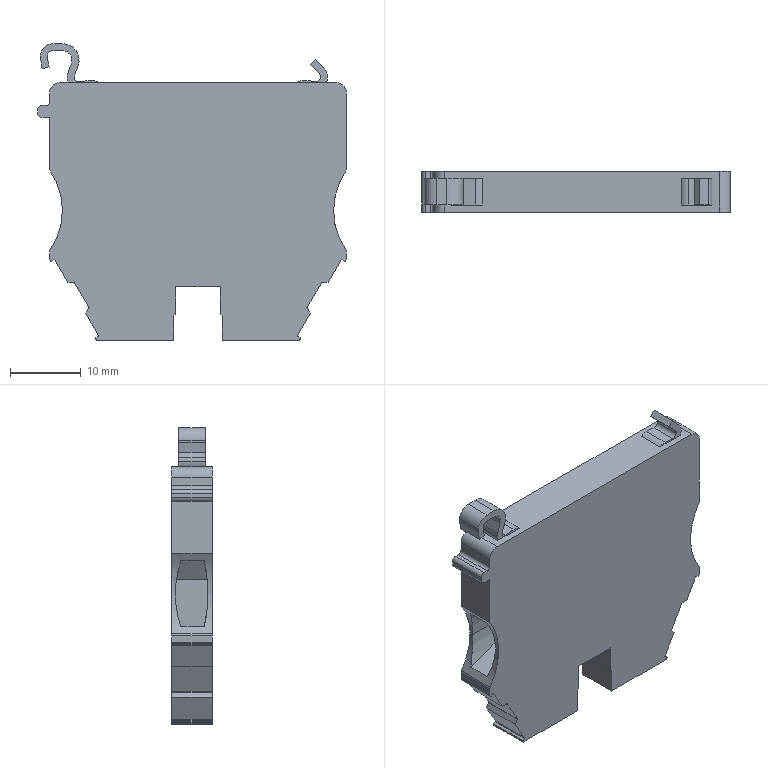Part | SolidWorks | features BaseBody 1 | 1 solid | 116 faces | box 43.7 x 5.75 x 42 mm | volume 7228 mm3 | plane 62 | cylinder 54 | commonest cylinder face diameters 0.2 x10 0.4 x4 0.6 x4 1.2 x4 3 x4 4 x4